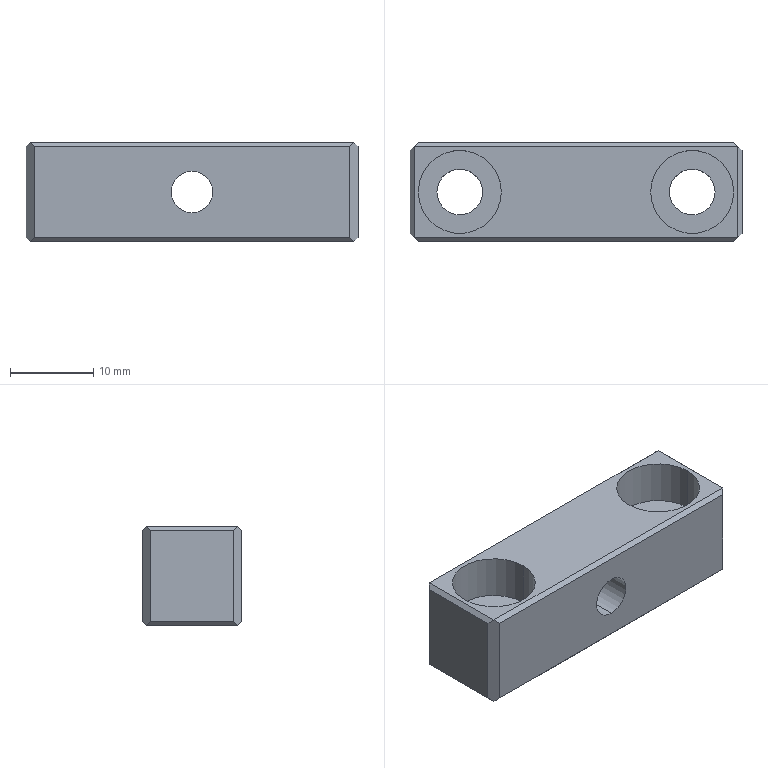Part | STEP file | 10000020605swp000-1 | 1 solid | 30 faces | box 40 x 12 x 12 mm | volume 4314 mm3 | plane 20 | cylinder 10 | commonest cylinder face diameters 5.5 x4 10 x4 5 x2
STEP:
#1=CARTESIAN_POINT('',(0.,6.,8.5));
#2=VERTEX_POINT('',#1);
#3=CARTESIAN_POINT('',(0.,6.,3.5));
#4=VERTEX_POINT('',#3);
#5=CARTESIAN_POINT('',(0.,6.,6.));
#6=DIRECTION('',(0.,-1.,0.));
#7=DIRECTION('',(0.,0.,-1.));
#8=AXIS2_PLACEMENT_3D('',#5,#6,#7);
#9=CIRCLE('',#8,2.5);
#10=EDGE_CURVE('',#2,#4,#9,.T.);
#11=ORIENTED_EDGE('',*,*,#10,.F.);
#12=CARTESIAN_POINT('',(0.,-6.,8.5));
#13=VERTEX_POINT('',#12);
#14=CARTESIAN_POINT('',(0.,-6.,8.5));
#15=DIRECTION('',(0.,-1.,0.));
#16=VECTOR('',#15,1000.);
#17=LINE('',#14,#16);
#18=EDGE_CURVE('',#2,#13,#17,.T.);
#19=ORIENTED_EDGE('',*,*,#18,.T.);
#20=CARTESIAN_POINT('',(0.,-6.,3.5));
#21=VERTEX_POINT('',#20);
#22=CARTESIAN_POINT('',(0.,-6.,6.));
#23=DIRECTION('',(0.,-1.,0.));
#24=DIRECTION('',(0.,0.,-1.));
#25=AXIS2_PLACEMENT_3D('',#22,#23,#24);
#26=CIRCLE('',#25,2.5);
#27=EDGE_CURVE('',#13,#21,#26,.T.);
#28=ORIENTED_EDGE('',*,*,#27,.T.);
#29=CARTESIAN_POINT('',(0.,-6.,3.5));
#30=DIRECTION('',(0.,-1.,0.));
#31=VECTOR('',#30,1000.);
#32=LINE('',#29,#31);
#33=EDGE_CURVE('',#4,#21,#32,.T.);
#34=ORIENTED_EDGE('',*,*,#33,.F.);
#35=EDGE_LOOP('',(#11,#19,#28,#34));
#36=FACE_OUTER_BOUND('',#35,.T.);
#37=CARTESIAN_POINT('',(0.,-6.,6.));
#38=DIRECTION('',(0.,-1.,0.));
#39=DIRECTION('',(0.,0.,-1.));
#40=AXIS2_PLACEMENT_3D('',#37,#38,#39);
#41=CYLINDRICAL_SURFACE('',#40,2.5);
#42=ADVANCED_FACE('',(#36),#41,.F.);
#43=CARTESIAN_POINT('',(-19.,0.,6.6));
#44=VERTEX_POINT('',#43);
#45=CARTESIAN_POINT('',(-9.,0.,6.6));
#46=VERTEX_POINT('',#45);
#47=CARTESIAN_POINT('',(-14.,0.,6.6));
#48=DIRECTION('',(0.,0.,1.));
#49=DIRECTION('',(1.,0.,0.));
#50=AXIS2_PLACEMENT_3D('',#47,#48,#49);
#51=CIRCLE('',#50,5.);
#52=EDGE_CURVE('',#44,#46,#51,.T.);
#53=ORIENTED_EDGE('',*,*,#52,.F.);
#54=CARTESIAN_POINT('',(-19.,0.,12.));
#55=VERTEX_POINT('',#54);
#56=CARTESIAN_POINT('',(-19.,0.,12.));
#57=DIRECTION('',(0.,0.,1.));
#58=VECTOR('',#57,1000.);
#59=LINE('',#56,#58);
#60=EDGE_CURVE('',#44,#55,#59,.T.);
#61=ORIENTED_EDGE('',*,*,#60,.T.);
#62=CARTESIAN_POINT('',(-9.,0.,12.));
#63=VERTEX_POINT('',#62);
#64=CARTESIAN_POINT('',(-14.,0.,12.));
#65=DIRECTION('',(0.,0.,1.));
#66=DIRECTION('',(1.,0.,0.));
#67=AXIS2_PLACEMENT_3D('',#64,#65,#66);
#68=CIRCLE('',#67,5.);
#69=EDGE_CURVE('',#55,#63,#68,.T.);
#70=ORIENTED_EDGE('',*,*,#69,.T.);
#71=CARTESIAN_POINT('',(-9.,0.,12.));
#72=DIRECTION('',(0.,0.,1.));
#73=VECTOR('',#72,1000.);
#74=LINE('',#71,#73);
#75=EDGE_CURVE('',#46,#63,#74,.T.);
#76=ORIENTED_EDGE('',*,*,#75,.F.);
#77=EDGE_LOOP('',(#53,#61,#70,#76));
#78=FACE_OUTER_BOUND('',#77,.T.);
#79=CARTESIAN_POINT('',(-14.,0.,12.));
#80=DIRECTION('',(0.,0.,1.));
#81=DIRECTION('',(1.,0.,0.));
#82=AXIS2_PLACEMENT_3D('',#79,#80,#81);
#83=CYLINDRICAL_SURFACE('',#82,5.);
#84=ADVANCED_FACE('',(#78),#83,.F.);
#85=CARTESIAN_POINT('',(-16.75,0.,0.));
#86=VERTEX_POINT('',#85);
#87=CARTESIAN_POINT('',(-11.25,0.,0.));
#88=VERTEX_POINT('',#87);
#89=CARTESIAN_POINT('',(-14.,0.,0.));
#90=DIRECTION('',(0.,0.,1.));
#91=DIRECTION('',(1.,0.,0.));
#92=AXIS2_PLACEMENT_3D('',#89,#90,#91);
#93=CIRCLE('',#92,2.75);
#94=EDGE_CURVE('',#86,#88,#93,.T.);
#95=ORIENTED_EDGE('',*,*,#94,.F.);
#96=CARTESIAN_POINT('',(-16.75,0.,6.6));
#97=VERTEX_POINT('',#96);
#98=CARTESIAN_POINT('',(-16.75,0.,12.));
#99=DIRECTION('',(0.,0.,1.));
#100=VECTOR('',#99,1000.);
#101=LINE('',#98,#100);
#102=EDGE_CURVE('',#86,#97,#101,.T.);
#103=ORIENTED_EDGE('',*,*,#102,.T.);
#104=CARTESIAN_POINT('',(-11.25,0.,6.6));
#105=VERTEX_POINT('',#104);
#106=CARTESIAN_POINT('',(-14.,0.,6.6));
#107=DIRECTION('',(0.,0.,1.));
#108=DIRECTION('',(1.,0.,0.));
#109=AXIS2_PLACEMENT_3D('',#106,#107,#108);
#110=CIRCLE('',#109,2.75);
#111=EDGE_CURVE('',#97,#105,#110,.T.);
#112=ORIENTED_EDGE('',*,*,#111,.T.);
#113=CARTESIAN_POINT('',(-11.25,0.,12.));
#114=DIRECTION('',(0.,0.,1.));
#115=VECTOR('',#114,1000.);
#116=LINE('',#113,#115);
#117=EDGE_CURVE('',#88,#105,#116,.T.);
#118=ORIENTED_EDGE('',*,*,#117,.F.);
#119=EDGE_LOOP('',(#95,#103,#112,#118));
#120=FACE_OUTER_BOUND('',#119,.T.);
#121=CARTESIAN_POINT('',(-14.,0.,12.));
#122=DIRECTION('',(0.,0.,1.));
#123=DIRECTION('',(1.,0.,0.));
#124=AXIS2_PLACEMENT_3D('',#121,#122,#123);
#125=CYLINDRICAL_SURFACE('',#124,2.75);
#126=ADVANCED_FACE('',(#120),#125,.F.);
#127=CARTESIAN_POINT('',(9.,0.,6.6));
#128=VERTEX_POINT('',#127);
#129=CARTESIAN_POINT('',(19.,0.,6.6));
#130=VERTEX_POINT('',#129);
#131=CARTESIAN_POINT('',(14.,0.,6.6));
#132=DIRECTION('',(0.,0.,1.));
#133=DIRECTION('',(1.,0.,0.));
#134=AXIS2_PLACEMENT_3D('',#131,#132,#133);
#135=CIRCLE('',#134,5.);
#136=EDGE_CURVE('',#128,#130,#135,.T.);
#137=ORIENTED_EDGE('',*,*,#136,.F.);
#138=CARTESIAN_POINT('',(9.,0.,12.));
#139=VERTEX_POINT('',#138);
#140=CARTESIAN_POINT('',(9.,0.,12.));
#141=DIRECTION('',(0.,0.,1.));
#142=VECTOR('',#141,1000.);
#143=LINE('',#140,#142);
#144=EDGE_CURVE('',#128,#139,#143,.T.);
#145=ORIENTED_EDGE('',*,*,#144,.T.);
#146=CARTESIAN_POINT('',(19.,0.,12.));
#147=VERTEX_POINT('',#146);
#148=CARTESIAN_POINT('',(14.,0.,12.));
#149=DIRECTION('',(0.,0.,1.));
#150=DIRECTION('',(1.,0.,0.));
#151=AXIS2_PLACEMENT_3D('',#148,#149,#150);
#152=CIRCLE('',#151,5.);
#153=EDGE_CURVE('',#139,#147,#152,.T.);
#154=ORIENTED_EDGE('',*,*,#153,.T.);
#155=CARTESIAN_POINT('',(19.,0.,12.));
#156=DIRECTION('',(0.,0.,1.));
#157=VECTOR('',#156,1000.);
#158=LINE('',#155,#157);
#159=EDGE_CURVE('',#130,#147,#158,.T.);
#160=ORIENTED_EDGE('',*,*,#159,.F.);
#161=EDGE_LOOP('',(#137,#145,#154,#160));
#162=FACE_OUTER_BOUND('',#161,.T.);
#163=CARTESIAN_POINT('',(14.,0.,12.));
#164=DIRECTION('',(0.,0.,1.));
#165=DIRECTION('',(1.,0.,0.));
#166=AXIS2_PLACEMENT_3D('',#163,#164,#165);
#167=CYLINDRICAL_SURFACE('',#166,5.);
#168=ADVANCED_FACE('',(#162),#167,.F.);
#169=CARTESIAN_POINT('',(11.25,0.,0.));
#170=VERTEX_POINT('',#169);
#171=CARTESIAN_POINT('',(16.75,0.,0.));
#172=VERTEX_POINT('',#171);
#173=CARTESIAN_POINT('',(14.,0.,0.));
#174=DIRECTION('',(0.,0.,1.));
#175=DIRECTION('',(1.,0.,0.));
#176=AXIS2_PLACEMENT_3D('',#173,#174,#175);
#177=CIRCLE('',#176,2.75);
#178=EDGE_CURVE('',#170,#172,#177,.T.);
#179=ORIENTED_EDGE('',*,*,#178,.F.);
#180=CARTESIAN_POINT('',(11.25,0.,6.6));
#181=VERTEX_POINT('',#180);
#182=CARTESIAN_POINT('',(11.25,0.,12.));
#183=DIRECTION('',(0.,0.,1.));
#184=VECTOR('',#183,1000.);
#185=LINE('',#182,#184);
#186=EDGE_CURVE('',#170,#181,#185,.T.);
#187=ORIENTED_EDGE('',*,*,#186,.T.);
#188=CARTESIAN_POINT('',(16.75,0.,6.6));
#189=VERTEX_POINT('',#188);
#190=CARTESIAN_POINT('',(14.,0.,6.6));
#191=DIRECTION('',(0.,0.,1.));
#192=DIRECTION('',(1.,0.,0.));
#193=AXIS2_PLACEMENT_3D('',#190,#191,#192);
#194=CIRCLE('',#193,2.75);
#195=EDGE_CURVE('',#181,#189,#194,.T.);
#196=ORIENTED_EDGE('',*,*,#195,.T.);
#197=CARTESIAN_POINT('',(16.75,0.,12.));
#198=DIRECTION('',(0.,0.,1.));
#199=VECTOR('',#198,1000.);
#200=LINE('',#197,#199);
#201=EDGE_CURVE('',#172,#189,#200,.T.);
#202=ORIENTED_EDGE('',*,*,#201,.F.);
#203=EDGE_LOOP('',(#179,#187,#196,#202));
#204=FACE_OUTER_BOUND('',#203,.T.);
#205=CARTESIAN_POINT('',(14.,0.,12.));
#206=DIRECTION('',(0.,0.,1.));
#207=DIRECTION('',(1.,0.,0.));
#208=AXIS2_PLACEMENT_3D('',#205,#206,#207);
#209=CYLINDRICAL_SURFACE('',#208,2.75);
#210=ADVANCED_FACE('',(#204),#209,.F.);
#211=CARTESIAN_POINT('',(-20.,5.,11.5));
#212=VERTEX_POINT('',#211);
#213=CARTESIAN_POINT('',(-20.,5.,0.5));
#214=VERTEX_POINT('',#213);
#215=CARTESIAN_POINT('',(-20.,5.,12.));
#216=DIRECTION('',(0.,0.,-1.));
#217=VECTOR('',#216,1000.);
#218=LINE('',#215,#217);
#219=EDGE_CURVE('',#212,#214,#218,.T.);
#220=ORIENTED_EDGE('',*,*,#219,.T.);
#221=CARTESIAN_POINT('',(-20.,-5.,0.5));
#222=VERTEX_POINT('',#221);
#223=CARTESIAN_POINT('',(-20.,6.,0.5));
#224=DIRECTION('',(0.,-1.,0.));
#225=VECTOR('',#224,1000.);
#226=LINE('',#223,#225);
#227=EDGE_CURVE('',#214,#222,#226,.T.);
#228=ORIENTED_EDGE('',*,*,#227,.T.);
#229=CARTESIAN_POINT('',(-20.,-5.,11.5));
#230=VERTEX_POINT('',#229);
#231=CARTESIAN_POINT('',(-20.,-5.,12.));
#232=DIRECTION('',(0.,0.,1.));
#233=VECTOR('',#232,1000.);
#234=LINE('',#231,#233);
#235=EDGE_CURVE('',#222,#230,#234,.T.);
#236=ORIENTED_EDGE('',*,*,#235,.T.);
#237=CARTESIAN_POINT('',(-20.,5.,11.5));
#238=DIRECTION('',(0.,1.,0.));
#239=VECTOR('',#238,1000.);
#240=LINE('',#237,#239);
#241=EDGE_CURVE('',#230,#212,#240,.T.);
#242=ORIENTED_EDGE('',*,*,#241,.T.);
#243=EDGE_LOOP('',(#220,#228,#236,#242));
#244=FACE_OUTER_BOUND('',#243,.T.);
#245=CARTESIAN_POINT('',(-20.,6.,12.));
#246=DIRECTION('',(1.,0.,0.));
#247=DIRECTION('',(0.,0.,-1.));
#248=AXIS2_PLACEMENT_3D('',#245,#246,#247);
#249=PLANE('',#248);
#250=ADVANCED_FACE('',(#244),#249,.F.);
#251=CARTESIAN_POINT('',(0.,-6.,6.));
#252=DIRECTION('',(0.,-1.,0.));
#253=DIRECTION('',(0.,0.,-1.));
#254=AXIS2_PLACEMENT_3D('',#251,#252,#253);
#255=CIRCLE('',#254,2.5);
#256=EDGE_CURVE('',#21,#13,#255,.T.);
#257=ORIENTED_EDGE('',*,*,#256,.F.);
#258=ORIENTED_EDGE('',*,*,#27,.F.);
#259=EDGE_LOOP('',(#257,#258));
#260=FACE_BOUND('',#259,.T.);
#261=CARTESIAN_POINT('',(-19.,-6.,11.5));
#262=VERTEX_POINT('',#261);
#263=CARTESIAN_POINT('',(-19.,-6.,0.5));
#264=VERTEX_POINT('',#263);
#265=CARTESIAN_POINT('',(-19.,-6.,12.));
#266=DIRECTION('',(0.,0.,-1.));
#267=VECTOR('',#266,1000.);
#268=LINE('',#265,#267);
#269=EDGE_CURVE('',#262,#264,#268,.T.);
#270=ORIENTED_EDGE('',*,*,#269,.T.);
#271=CARTESIAN_POINT('',(19.,-6.,0.5));
#272=VERTEX_POINT('',#271);
#273=CARTESIAN_POINT('',(-20.,-6.,0.5));
#274=DIRECTION('',(1.,0.,0.));
#275=VECTOR('',#274,1000.);
#276=LINE('',#273,#275);
#277=EDGE_CURVE('',#264,#272,#276,.T.);
#278=ORIENTED_EDGE('',*,*,#277,.T.);
#279=CARTESIAN_POINT('',(19.,-6.,11.5));
#280=VERTEX_POINT('',#279);
#281=CARTESIAN_POINT('',(19.,-6.,12.));
#282=DIRECTION('',(0.,0.,1.));
#283=VECTOR('',#282,1000.);
#284=LINE('',#281,#283);
#285=EDGE_CURVE('',#272,#280,#284,.T.);
#286=ORIENTED_EDGE('',*,*,#285,.T.);
#287=CARTESIAN_POINT('',(-19.,-6.,11.5));
#288=DIRECTION('',(-1.,0.,0.));
#289=VECTOR('',#288,1000.);
#290=LINE('',#287,#289);
#291=EDGE_CURVE('',#280,#262,#290,.T.);
#292=ORIENTED_EDGE('',*,*,#291,.T.);
#293=EDGE_LOOP('',(#270,#278,#286,#292));
#294=FACE_OUTER_BOUND('',#293,.T.);
#295=CARTESIAN_POINT('',(-20.,-6.,12.));
#296=DIRECTION('',(0.,1.,0.));
#297=DIRECTION('',(0.,0.,1.));
#298=AXIS2_PLACEMENT_3D('',#295,#296,#297);
#299=PLANE('',#298);
#300=ADVANCED_FACE('',(#260,#294),#299,.F.);
#301=CARTESIAN_POINT('',(20.,-5.,11.5));
#302=VERTEX_POINT('',#301);
#303=CARTESIAN_POINT('',(20.,-5.,0.5));
#304=VERTEX_POINT('',#303);
#305=CARTESIAN_POINT('',(20.,-5.,12.));
#306=DIRECTION('',(0.,0.,-1.));
#307=VECTOR('',#306,1000.);
#308=LINE('',#305,#307);
#309=EDGE_CURVE('',#302,#304,#308,.T.);
#310=ORIENTED_EDGE('',*,*,#309,.T.);
#311=CARTESIAN_POINT('',(20.,5.,0.5));
#312=VERTEX_POINT('',#311);
#313=CARTESIAN_POINT('',(20.,6.,0.5));
#314=DIRECTION('',(0.,1.,0.));
#315=VECTOR('',#314,1000.);
#316=LINE('',#313,#315);
#317=EDGE_CURVE('',#304,#312,#316,.T.);
#318=ORIENTED_EDGE('',*,*,#317,.T.);
#319=CARTESIAN_POINT('',(20.,5.,11.5));
#320=VERTEX_POINT('',#319);
#321=CARTESIAN_POINT('',(20.,5.,12.));
#322=DIRECTION('',(0.,0.,1.));
#323=VECTOR('',#322,1000.);
#324=LINE('',#321,#323);
#325=EDGE_CURVE('',#312,#320,#324,.T.);
#326=ORIENTED_EDGE('',*,*,#325,.T.);
#327=CARTESIAN_POINT('',(20.,-5.,11.5));
#328=DIRECTION('',(0.,-1.,0.));
#329=VECTOR('',#328,1000.);
#330=LINE('',#327,#329);
#331=EDGE_CURVE('',#320,#302,#330,.T.);
#332=ORIENTED_EDGE('',*,*,#331,.T.);
#333=EDGE_LOOP('',(#310,#318,#326,#332));
#334=FACE_OUTER_BOUND('',#333,.T.);
#335=CARTESIAN_POINT('',(20.,6.,12.));
#336=DIRECTION('',(-1.,0.,0.));
#337=DIRECTION('',(0.,0.,1.));
#338=AXIS2_PLACEMENT_3D('',#335,#336,#337);
#339=PLANE('',#338);
#340=ADVANCED_FACE('',(#334),#339,.F.);
#341=CARTESIAN_POINT('',(0.,6.,6.));
#342=DIRECTION('',(0.,-1.,0.));
#343=DIRECTION('',(0.,0.,-1.));
#344=AXIS2_PLACEMENT_3D('',#341,#342,#343);
#345=CIRCLE('',#344,2.5);
#346=EDGE_CURVE('',#4,#2,#345,.T.);
#347=ORIENTED_EDGE('',*,*,#346,.T.);
#348=ORIENTED_EDGE('',*,*,#10,.T.);
#349=EDGE_LOOP('',(#347,#348));
#350=FACE_BOUND('',#349,.T.);
#351=CARTESIAN_POINT('',(19.,6.,11.5));
#352=VERTEX_POINT('',#351);
#353=CARTESIAN_POINT('',(19.,6.,0.5));
#354=VERTEX_POINT('',#353);
#355=CARTESIAN_POINT('',(19.,6.,12.));
#356=DIRECTION('',(0.,0.,-1.));
#357=VECTOR('',#356,1000.);
#358=LINE('',#355,#357);
#359=EDGE_CURVE('',#352,#354,#358,.T.);
#360=ORIENTED_EDGE('',*,*,#359,.T.);
#361=CARTESIAN_POINT('',(-19.,6.,0.5));
#362=VERTEX_POINT('',#361);
#363=CARTESIAN_POINT('',(-20.,6.,0.5));
#364=DIRECTION('',(-1.,0.,0.));
#365=VECTOR('',#364,1000.);
#366=LINE('',#363,#365);
#367=EDGE_CURVE('',#354,#362,#366,.T.);
#368=ORIENTED_EDGE('',*,*,#367,.T.);
#369=CARTESIAN_POINT('',(-19.,6.,11.5));
#370=VERTEX_POINT('',#369);
#371=CARTESIAN_POINT('',(-19.,6.,12.));
#372=DIRECTION('',(0.,0.,1.));
#373=VECTOR('',#372,1000.);
#374=LINE('',#371,#373);
#375=EDGE_CURVE('',#362,#370,#374,.T.);
#376=ORIENTED_EDGE('',*,*,#375,.T.);
#377=CARTESIAN_POINT('',(19.,6.,11.5));
#378=DIRECTION('',(1.,0.,0.));
#379=VECTOR('',#378,1000.);
#380=LINE('',#377,#379);
#381=EDGE_CURVE('',#370,#352,#380,.T.);
#382=ORIENTED_EDGE('',*,*,#381,.T.);
#383=EDGE_LOOP('',(#360,#368,#376,#382));
#384=FACE_OUTER_BOUND('',#383,.T.);
#385=CARTESIAN_POINT('',(-20.,6.,12.));
#386=DIRECTION('',(0.,-1.,0.));
#387=DIRECTION('',(0.,0.,-1.));
#388=AXIS2_PLACEMENT_3D('',#385,#386,#387);
#389=PLANE('',#388);
#390=ADVANCED_FACE('',(#350,#384),#389,.F.);
#391=CARTESIAN_POINT('',(-14.,0.,12.));
#392=DIRECTION('',(0.,0.,1.));
#393=DIRECTION('',(1.,0.,0.));
#394=AXIS2_PLACEMENT_3D('',#391,#392,#393);
#395=CIRCLE('',#394,5.);
#396=EDGE_CURVE('',#63,#55,#395,.T.);
#397=ORIENTED_EDGE('',*,*,#396,.F.);
#398=ORIENTED_EDGE('',*,*,#69,.F.);
#399=EDGE_LOOP('',(#397,#398));
#400=FACE_BOUND('',#399,.T.);
#401=CARTESIAN_POINT('',(14.,0.,12.));
#402=DIRECTION('',(0.,0.,1.));
#403=DIRECTION('',(1.,0.,0.));
#404=AXIS2_PLACEMENT_3D('',#401,#402,#403);
#405=CIRCLE('',#404,5.);
#406=EDGE_CURVE('',#147,#139,#405,.T.);
#407=ORIENTED_EDGE('',*,*,#406,.F.);
#408=ORIENTED_EDGE('',*,*,#153,.F.);
#409=EDGE_LOOP('',(#407,#408));
#410=FACE_BOUND('',#409,.T.);
#411=CARTESIAN_POINT('',(19.5,5.5,12.));
#412=VERTEX_POINT('',#411);
#413=CARTESIAN_POINT('',(-19.5,5.5,12.));
#414=VERTEX_POINT('',#413);
#415=CARTESIAN_POINT('',(-19.,5.5,12.));
#416=DIRECTION('',(-1.,0.,0.));
#417=VECTOR('',#416,1000.);
#418=LINE('',#415,#417);
#419=EDGE_CURVE('',#412,#414,#418,.T.);
#420=ORIENTED_EDGE('',*,*,#419,.T.);
#421=CARTESIAN_POINT('',(-19.5,-5.5,12.));
#422=VERTEX_POINT('',#421);
#423=CARTESIAN_POINT('',(-19.5,-5.,12.));
#424=DIRECTION('',(0.,-1.,0.));
#425=VECTOR('',#424,1000.);
#426=LINE('',#423,#425);
#427=EDGE_CURVE('',#414,#422,#426,.T.);
#428=ORIENTED_EDGE('',*,*,#427,.T.);
#429=CARTESIAN_POINT('',(19.5,-5.5,12.));
#430=VERTEX_POINT('',#429);
#431=CARTESIAN_POINT('',(19.,-5.5,12.));
#432=DIRECTION('',(1.,0.,0.));
#433=VECTOR('',#432,1000.);
#434=LINE('',#431,#433);
#435=EDGE_CURVE('',#422,#430,#434,.T.);
#436=ORIENTED_EDGE('',*,*,#435,.T.);
#437=CARTESIAN_POINT('',(19.5,5.,12.));
#438=DIRECTION('',(0.,1.,0.));
#439=VECTOR('',#438,1000.);
#440=LINE('',#437,#439);
#441=EDGE_CURVE('',#430,#412,#440,.T.);
#442=ORIENTED_EDGE('',*,*,#441,.T.);
#443=EDGE_LOOP('',(#420,#428,#436,#442));
#444=FACE_OUTER_BOUND('',#443,.T.);
#445=CARTESIAN_POINT('',(0.,0.,12.));
#446=DIRECTION('',(0.,0.,1.));
#447=DIRECTION('',(1.,0.,0.));
#448=AXIS2_PLACEMENT_3D('',#445,#446,#447);
#449=PLANE('',#448);
#450=ADVANCED_FACE('',(#400,#410,#444),#449,.T.);
#451=CARTESIAN_POINT('',(-14.,0.,0.));
#452=DIRECTION('',(0.,0.,1.));
#453=DIRECTION('',(1.,0.,0.));
#454=AXIS2_PLACEMENT_3D('',#451,#452,#453);
#455=CIRCLE('',#454,2.75);
#456=EDGE_CURVE('',#88,#86,#455,.T.);
#457=ORIENTED_EDGE('',*,*,#456,.T.);
#458=ORIENTED_EDGE('',*,*,#94,.T.);
#459=EDGE_LOOP('',(#457,#458));
#460=FACE_BOUND('',#459,.T.);
#461=CARTESIAN_POINT('',(14.,0.,0.));
#462=DIRECTION('',(0.,0.,1.));
#463=DIRECTION('',(1.,0.,0.));
#464=AXIS2_PLACEMENT_3D('',#461,#462,#463);
#465=CIRCLE('',#464,2.75);
#466=EDGE_CURVE('',#172,#170,#465,.T.);
#467=ORIENTED_EDGE('',*,*,#466,.T.);
#468=ORIENTED_EDGE('',*,*,#178,.T.);
#469=EDGE_LOOP('',(#467,#468));
#470=FACE_BOUND('',#469,.T.);
#471=CARTESIAN_POINT('',(19.5,5.5,0.));
#472=VERTEX_POINT('',#471);
#473=CARTESIAN_POINT('',(19.5,-5.5,0.));
#474=VERTEX_POINT('',#473);
#475=CARTESIAN_POINT('',(19.5,0.,0.));
#476=DIRECTION('',(0.,-1.,0.));
#477=VECTOR('',#476,1000.);
#478=LINE('',#475,#477);
#479=EDGE_CURVE('',#472,#474,#478,.T.);
#480=ORIENTED_EDGE('',*,*,#479,.T.);
#481=CARTESIAN_POINT('',(-19.5,-5.5,0.));
#482=VERTEX_POINT('',#481);
#483=CARTESIAN_POINT('',(0.,-5.5,0.));
#484=DIRECTION('',(-1.,0.,0.));
#485=VECTOR('',#484,1000.);
#486=LINE('',#483,#485);
#487=EDGE_CURVE('',#474,#482,#486,.T.);
#488=ORIENTED_EDGE('',*,*,#487,.T.);
#489=CARTESIAN_POINT('',(-19.5,5.5,0.));
#490=VERTEX_POINT('',#489);
#491=CARTESIAN_POINT('',(-19.5,0.,0.));
#492=DIRECTION('',(0.,1.,0.));
#493=VECTOR('',#492,1000.);
#494=LINE('',#491,#493);
#495=EDGE_CURVE('',#482,#490,#494,.T.);
#496=ORIENTED_EDGE('',*,*,#495,.T.);
#497=CARTESIAN_POINT('',(0.,5.5,0.));
#498=DIRECTION('',(1.,0.,0.));
#499=VECTOR('',#498,1000.);
#500=LINE('',#497,#499);
#501=EDGE_CURVE('',#490,#472,#500,.T.);
#502=ORIENTED_EDGE('',*,*,#501,.T.);
#503=EDGE_LOOP('',(#480,#488,#496,#502));
#504=FACE_OUTER_BOUND('',#503,.T.);
#505=CARTESIAN_POINT('',(0.,0.,0.));
#506=DIRECTION('',(0.,0.,1.));
#507=DIRECTION('',(1.,0.,0.));
#508=AXIS2_PLACEMENT_3D('',#505,#506,#507);
#509=PLANE('',#508);
#510=ADVANCED_FACE('',(#460,#470,#504),#509,.F.);
#511=ORIENTED_EDGE('',*,*,#186,.F.);
#512=ORIENTED_EDGE('',*,*,#466,.F.);
#513=ORIENTED_EDGE('',*,*,#201,.T.);
#514=CARTESIAN_POINT('',(14.,0.,6.6));
#515=DIRECTION('',(0.,0.,1.));
#516=DIRECTION('',(1.,0.,0.));
#517=AXIS2_PLACEMENT_3D('',#514,#515,#516);
#518=CIRCLE('',#517,2.75);
#519=EDGE_CURVE('',#189,#181,#518,.T.);
#520=ORIENTED_EDGE('',*,*,#519,.T.);
#521=EDGE_LOOP('',(#511,#512,#513,#520));
#522=FACE_OUTER_BOUND('',#521,.T.);
#523=CARTESIAN_POINT('',(14.,0.,12.));
#524=DIRECTION('',(0.,0.,1.));
#525=DIRECTION('',(1.,0.,0.));
#526=AXIS2_PLACEMENT_3D('',#523,#524,#525);
#527=CYLINDRICAL_SURFACE('',#526,2.75);
#528=ADVANCED_FACE('',(#522),#527,.F.);
#529=ORIENTED_EDGE('',*,*,#519,.F.);
#530=ORIENTED_EDGE('',*,*,#195,.F.);
#531=EDGE_LOOP('',(#529,#530));
#532=FACE_BOUND('',#531,.T.);
#533=CARTESIAN_POINT('',(14.,0.,6.6));
#534=DIRECTION('',(0.,0.,1.));
#535=DIRECTION('',(1.,0.,0.));
#536=AXIS2_PLACEMENT_3D('',#533,#534,#535);
#537=CIRCLE('',#536,5.);
#538=EDGE_CURVE('',#130,#128,#537,.T.);
#539=ORIENTED_EDGE('',*,*,#538,.T.);
#540=ORIENTED_EDGE('',*,*,#136,.T.);
#541=EDGE_LOOP('',(#539,#540));
#542=FACE_OUTER_BOUND('',#541,.T.);
#543=CARTESIAN_POINT('',(16.75,0.,6.6));
#544=DIRECTION('',(0.,0.,-1.));
#545=DIRECTION('',(-1.,0.,0.));
#546=AXIS2_PLACEMENT_3D('',#543,#544,#545);
#547=PLANE('',#546);
#548=ADVANCED_FACE('',(#532,#542),#547,.F.);
#549=ORIENTED_EDGE('',*,*,#144,.F.);
#550=ORIENTED_EDGE('',*,*,#538,.F.);
#551=ORIENTED_EDGE('',*,*,#159,.T.);
#552=ORIENTED_EDGE('',*,*,#406,.T.);
#553=EDGE_LOOP('',(#549,#550,#551,#552));
#554=FACE_OUTER_BOUND('',#553,.T.);
#555=CARTESIAN_POINT('',(14.,0.,12.));
#556=DIRECTION('',(0.,0.,1.));
#557=DIRECTION('',(1.,0.,0.));
#558=AXIS2_PLACEMENT_3D('',#555,#556,#557);
#559=CYLINDRICAL_SURFACE('',#558,5.);
#560=ADVANCED_FACE('',(#554),#559,.F.);
#561=ORIENTED_EDGE('',*,*,#102,.F.);
#562=ORIENTED_EDGE('',*,*,#456,.F.);
#563=ORIENTED_EDGE('',*,*,#117,.T.);
#564=CARTESIAN_POINT('',(-14.,0.,6.6));
#565=DIRECTION('',(0.,0.,1.));
#566=DIRECTION('',(1.,0.,0.));
#567=AXIS2_PLACEMENT_3D('',#564,#565,#566);
#568=CIRCLE('',#567,2.75);
#569=EDGE_CURVE('',#105,#97,#568,.T.);
#570=ORIENTED_EDGE('',*,*,#569,.T.);
#571=EDGE_LOOP('',(#561,#562,#563,#570));
#572=FACE_OUTER_BOUND('',#571,.T.);
#573=CARTESIAN_POINT('',(-14.,0.,12.));
#574=DIRECTION('',(0.,0.,1.));
#575=DIRECTION('',(1.,0.,0.));
#576=AXIS2_PLACEMENT_3D('',#573,#574,#575);
#577=CYLINDRICAL_SURFACE('',#576,2.75);
#578=ADVANCED_FACE('',(#572),#577,.F.);
#579=ORIENTED_EDGE('',*,*,#569,.F.);
#580=ORIENTED_EDGE('',*,*,#111,.F.);
#581=EDGE_LOOP('',(#579,#580));
#582=FACE_BOUND('',#581,.T.);
#583=CARTESIAN_POINT('',(-14.,0.,6.6));
#584=DIRECTION('',(0.,0.,1.));
#585=DIRECTION('',(1.,0.,0.));
#586=AXIS2_PLACEMENT_3D('',#583,#584,#585);
#587=CIRCLE('',#586,5.);
#588=EDGE_CURVE('',#46,#44,#587,.T.);
#589=ORIENTED_EDGE('',*,*,#588,.T.);
#590=ORIENTED_EDGE('',*,*,#52,.T.);
#591=EDGE_LOOP('',(#589,#590));
#592=FACE_OUTER_BOUND('',#591,.T.);
#593=CARTESIAN_POINT('',(-11.25,0.,6.6));
#594=DIRECTION('',(0.,0.,-1.));
#595=DIRECTION('',(-1.,0.,0.));
#596=AXIS2_PLACEMENT_3D('',#593,#594,#595);
#597=PLANE('',#596);
#598=ADVANCED_FACE('',(#582,#592),#597,.F.);
#599=ORIENTED_EDGE('',*,*,#60,.F.);
#600=ORIENTED_EDGE('',*,*,#588,.F.);
#601=ORIENTED_EDGE('',*,*,#75,.T.);
#602=ORIENTED_EDGE('',*,*,#396,.T.);
#603=EDGE_LOOP('',(#599,#600,#601,#602));
#604=FACE_OUTER_BOUND('',#603,.T.);
#605=CARTESIAN_POINT('',(-14.,0.,12.));
#606=DIRECTION('',(0.,0.,1.));
#607=DIRECTION('',(1.,0.,0.));
#608=AXIS2_PLACEMENT_3D('',#605,#606,#607);
#609=CYLINDRICAL_SURFACE('',#608,5.);
#610=ADVANCED_FACE('',(#604),#609,.F.);
#611=ORIENTED_EDGE('',*,*,#18,.F.);
#612=ORIENTED_EDGE('',*,*,#346,.F.);
#613=ORIENTED_EDGE('',*,*,#33,.T.);
#614=ORIENTED_EDGE('',*,*,#256,.T.);
#615=EDGE_LOOP('',(#611,#612,#613,#614));
#616=FACE_OUTER_BOUND('',#615,.T.);
#617=CARTESIAN_POINT('',(0.,-6.,6.));
#618=DIRECTION('',(0.,-1.,0.));
#619=DIRECTION('',(0.,0.,-1.));
#620=AXIS2_PLACEMENT_3D('',#617,#618,#619);
#621=CYLINDRICAL_SURFACE('',#620,2.5);
#622=ADVANCED_FACE('',(#616),#621,.F.);
#623=ORIENTED_EDGE('',*,*,#285,.F.);
#624=CARTESIAN_POINT('',(15.833,-9.167,3.667));
#625=DIRECTION('',(0.5774,0.5774,-0.5774));
#626=VECTOR('',#625,1000.);
#627=LINE('',#624,#626);
#628=EDGE_CURVE('',#272,#474,#627,.T.);
#629=ORIENTED_EDGE('',*,*,#628,.T.);
#630=CARTESIAN_POINT('',(23.833,-1.167,4.333));
#631=DIRECTION('',(0.5774,0.5774,0.5774));
#632=VECTOR('',#631,1000.);
#633=LINE('',#630,#632);
#634=EDGE_CURVE('',#474,#304,#633,.T.);
#635=ORIENTED_EDGE('',*,*,#634,.T.);
#636=ORIENTED_EDGE('',*,*,#309,.F.);
#637=CARTESIAN_POINT('',(19.833,-5.167,11.667));
#638=DIRECTION('',(-0.5774,-0.5774,0.5774));
#639=VECTOR('',#638,1000.);
#640=LINE('',#637,#639);
#641=EDGE_CURVE('',#302,#430,#640,.T.);
#642=ORIENTED_EDGE('',*,*,#641,.T.);
#643=CARTESIAN_POINT('',(19.833,-5.167,12.333));
#644=DIRECTION('',(-0.5774,-0.5774,-0.5774));
#645=VECTOR('',#644,1000.);
#646=LINE('',#643,#645);
#647=EDGE_CURVE('',#430,#280,#646,.T.);
#648=ORIENTED_EDGE('',*,*,#647,.T.);
#649=EDGE_LOOP('',(#623,#629,#635,#636,#642,#648));
#650=FACE_OUTER_BOUND('',#649,.T.);
#651=CARTESIAN_POINT('',(20.,-5.,12.));
#652=DIRECTION('',(-0.7071,0.7071,0.));
#653=DIRECTION('',(0.,0.,-1.));
#654=AXIS2_PLACEMENT_3D('',#651,#652,#653);
#655=PLANE('',#654);
#656=ADVANCED_FACE('',(#650),#655,.F.);
#657=ORIENTED_EDGE('',*,*,#325,.F.);
#658=CARTESIAN_POINT('',(23.167,1.833,3.667));
#659=DIRECTION('',(-0.5774,0.5774,-0.5774));
#660=VECTOR('',#659,1000.);
#661=LINE('',#658,#660);
#662=EDGE_CURVE('',#312,#472,#661,.T.);
#663=ORIENTED_EDGE('',*,*,#662,.T.);
#664=CARTESIAN_POINT('',(15.167,9.833,4.333));
#665=DIRECTION('',(-0.5774,0.5774,0.5774));
#666=VECTOR('',#665,1000.);
#667=LINE('',#664,#666);
#668=EDGE_CURVE('',#472,#354,#667,.T.);
#669=ORIENTED_EDGE('',*,*,#668,.T.);
#670=ORIENTED_EDGE('',*,*,#359,.F.);
#671=CARTESIAN_POINT('',(19.167,5.833,11.667));
#672=DIRECTION('',(0.5774,-0.5774,0.5774));
#673=VECTOR('',#672,1000.);
#674=LINE('',#671,#673);
#675=EDGE_CURVE('',#352,#412,#674,.T.);
#676=ORIENTED_EDGE('',*,*,#675,.T.);
#677=CARTESIAN_POINT('',(19.167,5.833,12.333));
#678=DIRECTION('',(0.5774,-0.5774,-0.5774));
#679=VECTOR('',#678,1000.);
#680=LINE('',#677,#679);
#681=EDGE_CURVE('',#412,#320,#680,.T.);
#682=ORIENTED_EDGE('',*,*,#681,.T.);
#683=EDGE_LOOP('',(#657,#663,#669,#670,#676,#682));
#684=FACE_OUTER_BOUND('',#683,.T.);
#685=CARTESIAN_POINT('',(19.,6.,12.));
#686=DIRECTION('',(-0.7071,-0.7071,0.));
#687=DIRECTION('',(0.,0.,-1.));
#688=AXIS2_PLACEMENT_3D('',#685,#686,#687);
#689=PLANE('',#688);
#690=ADVANCED_FACE('',(#684),#689,.F.);
#691=CARTESIAN_POINT('',(-23.167,-1.833,3.667));
#692=DIRECTION('',(0.5774,-0.5774,-0.5774));
#693=VECTOR('',#692,1000.);
#694=LINE('',#691,#693);
#695=EDGE_CURVE('',#222,#482,#694,.T.);
#696=ORIENTED_EDGE('',*,*,#695,.T.);
#697=CARTESIAN_POINT('',(-15.167,-9.833,4.333));
#698=DIRECTION('',(0.5774,-0.5774,0.5774));
#699=VECTOR('',#698,1000.);
#700=LINE('',#697,#699);
#701=EDGE_CURVE('',#482,#264,#700,.T.);
#702=ORIENTED_EDGE('',*,*,#701,.T.);
#703=ORIENTED_EDGE('',*,*,#269,.F.);
#704=CARTESIAN_POINT('',(-19.167,-5.833,11.667));
#705=DIRECTION('',(-0.5774,0.5774,0.5774));
#706=VECTOR('',#705,1000.);
#707=LINE('',#704,#706);
#708=EDGE_CURVE('',#262,#422,#707,.T.);
#709=ORIENTED_EDGE('',*,*,#708,.T.);
#710=CARTESIAN_POINT('',(-19.167,-5.833,12.333));
#711=DIRECTION('',(-0.5774,0.5774,-0.5774));
#712=VECTOR('',#711,1000.);
#713=LINE('',#710,#712);
#714=EDGE_CURVE('',#422,#230,#713,.T.);
#715=ORIENTED_EDGE('',*,*,#714,.T.);
#716=ORIENTED_EDGE('',*,*,#235,.F.);
#717=EDGE_LOOP('',(#696,#702,#703,#709,#715,#716));
#718=FACE_OUTER_BOUND('',#717,.T.);
#719=CARTESIAN_POINT('',(-19.,-6.,12.));
#720=DIRECTION('',(0.7071,0.7071,0.));
#721=DIRECTION('',(0.,0.,-1.));
#722=AXIS2_PLACEMENT_3D('',#719,#720,#721);
#723=PLANE('',#722);
#724=ADVANCED_FACE('',(#718),#723,.F.);
#725=CARTESIAN_POINT('',(-15.833,9.167,3.667));
#726=DIRECTION('',(-0.5774,-0.5774,-0.5774));
#727=VECTOR('',#726,1000.);
#728=LINE('',#725,#727);
#729=EDGE_CURVE('',#362,#490,#728,.T.);
#730=ORIENTED_EDGE('',*,*,#729,.T.);
#731=CARTESIAN_POINT('',(-23.833,1.167,4.333));
#732=DIRECTION('',(-0.5774,-0.5774,0.5774));
#733=VECTOR('',#732,1000.);
#734=LINE('',#731,#733);
#735=EDGE_CURVE('',#490,#214,#734,.T.);
#736=ORIENTED_EDGE('',*,*,#735,.T.);
#737=ORIENTED_EDGE('',*,*,#219,.F.);
#738=CARTESIAN_POINT('',(-19.833,5.167,11.667));
#739=DIRECTION('',(0.5774,0.5774,0.5774));
#740=VECTOR('',#739,1000.);
#741=LINE('',#738,#740);
#742=EDGE_CURVE('',#212,#414,#741,.T.);
#743=ORIENTED_EDGE('',*,*,#742,.T.);
#744=CARTESIAN_POINT('',(-19.833,5.167,12.333));
#745=DIRECTION('',(0.5774,0.5774,-0.5774));
#746=VECTOR('',#745,1000.);
#747=LINE('',#744,#746);
#748=EDGE_CURVE('',#414,#370,#747,.T.);
#749=ORIENTED_EDGE('',*,*,#748,.T.);
#750=ORIENTED_EDGE('',*,*,#375,.F.);
#751=EDGE_LOOP('',(#730,#736,#737,#743,#749,#750));
#752=FACE_OUTER_BOUND('',#751,.T.);
#753=CARTESIAN_POINT('',(-20.,5.,12.));
#754=DIRECTION('',(0.7071,-0.7071,0.));
#755=DIRECTION('',(0.,0.,-1.));
#756=AXIS2_PLACEMENT_3D('',#753,#754,#755);
#757=PLANE('',#756);
#758=ADVANCED_FACE('',(#752),#757,.F.);
#759=ORIENTED_EDGE('',*,*,#701,.F.);
#760=ORIENTED_EDGE('',*,*,#487,.F.);
#761=ORIENTED_EDGE('',*,*,#628,.F.);
#762=ORIENTED_EDGE('',*,*,#277,.F.);
#763=EDGE_LOOP('',(#759,#760,#761,#762));
#764=FACE_OUTER_BOUND('',#763,.T.);
#765=CARTESIAN_POINT('',(-20.,-6.,0.5));
#766=DIRECTION('',(0.,0.7071,0.7071));
#767=DIRECTION('',(1.,0.,0.));
#768=AXIS2_PLACEMENT_3D('',#765,#766,#767);
#769=PLANE('',#768);
#770=ADVANCED_FACE('',(#764),#769,.F.);
#771=ORIENTED_EDGE('',*,*,#634,.F.);
#772=ORIENTED_EDGE('',*,*,#479,.F.);
#773=ORIENTED_EDGE('',*,*,#662,.F.);
#774=ORIENTED_EDGE('',*,*,#317,.F.);
#775=EDGE_LOOP('',(#771,#772,#773,#774));
#776=FACE_OUTER_BOUND('',#775,.T.);
#777=CARTESIAN_POINT('',(20.,6.,0.5));
#778=DIRECTION('',(-0.7071,0.,0.7071));
#779=DIRECTION('',(0.,1.,0.));
#780=AXIS2_PLACEMENT_3D('',#777,#778,#779);
#781=PLANE('',#780);
#782=ADVANCED_FACE('',(#776),#781,.F.);
#783=ORIENTED_EDGE('',*,*,#735,.F.);
#784=ORIENTED_EDGE('',*,*,#495,.F.);
#785=ORIENTED_EDGE('',*,*,#695,.F.);
#786=ORIENTED_EDGE('',*,*,#227,.F.);
#787=EDGE_LOOP('',(#783,#784,#785,#786));
#788=FACE_OUTER_BOUND('',#787,.T.);
#789=CARTESIAN_POINT('',(-20.,6.,0.5));
#790=DIRECTION('',(0.7071,0.,0.7071));
#791=DIRECTION('',(0.,-1.,0.));
#792=AXIS2_PLACEMENT_3D('',#789,#790,#791);
#793=PLANE('',#792);
#794=ADVANCED_FACE('',(#788),#793,.F.);
#795=ORIENTED_EDGE('',*,*,#668,.F.);
#796=ORIENTED_EDGE('',*,*,#501,.F.);
#797=ORIENTED_EDGE('',*,*,#729,.F.);
#798=ORIENTED_EDGE('',*,*,#367,.F.);
#799=EDGE_LOOP('',(#795,#796,#797,#798));
#800=FACE_OUTER_BOUND('',#799,.T.);
#801=CARTESIAN_POINT('',(-20.,6.,0.5));
#802=DIRECTION('',(0.,-0.7071,0.7071));
#803=DIRECTION('',(-1.,0.,0.));
#804=AXIS2_PLACEMENT_3D('',#801,#802,#803);
#805=PLANE('',#804);
#806=ADVANCED_FACE('',(#800),#805,.F.);
#807=ORIENTED_EDGE('',*,*,#742,.F.);
#808=ORIENTED_EDGE('',*,*,#241,.F.);
#809=ORIENTED_EDGE('',*,*,#714,.F.);
#810=ORIENTED_EDGE('',*,*,#427,.F.);
#811=EDGE_LOOP('',(#807,#808,#809,#810));
#812=FACE_OUTER_BOUND('',#811,.T.);
#813=CARTESIAN_POINT('',(-19.5,0.,12.));
#814=DIRECTION('',(-0.7071,0.,0.7071));
#815=DIRECTION('',(0.,1.,0.));
#816=AXIS2_PLACEMENT_3D('',#813,#814,#815);
#817=PLANE('',#816);
#818=ADVANCED_FACE('',(#812),#817,.T.);
#819=ORIENTED_EDGE('',*,*,#708,.F.);
#820=ORIENTED_EDGE('',*,*,#291,.F.);
#821=ORIENTED_EDGE('',*,*,#647,.F.);
#822=ORIENTED_EDGE('',*,*,#435,.F.);
#823=EDGE_LOOP('',(#819,#820,#821,#822));
#824=FACE_OUTER_BOUND('',#823,.T.);
#825=CARTESIAN_POINT('',(0.,-5.5,12.));
#826=DIRECTION('',(0.,-0.7071,0.7071));
#827=DIRECTION('',(-1.,0.,0.));
#828=AXIS2_PLACEMENT_3D('',#825,#826,#827);
#829=PLANE('',#828);
#830=ADVANCED_FACE('',(#824),#829,.T.);
#831=ORIENTED_EDGE('',*,*,#675,.F.);
#832=ORIENTED_EDGE('',*,*,#381,.F.);
#833=ORIENTED_EDGE('',*,*,#748,.F.);
#834=ORIENTED_EDGE('',*,*,#419,.F.);
#835=EDGE_LOOP('',(#831,#832,#833,#834));
#836=FACE_OUTER_BOUND('',#835,.T.);
#837=CARTESIAN_POINT('',(0.,5.5,12.));
#838=DIRECTION('',(0.,0.7071,0.7071));
#839=DIRECTION('',(1.,0.,0.));
#840=AXIS2_PLACEMENT_3D('',#837,#838,#839);
#841=PLANE('',#840);
#842=ADVANCED_FACE('',(#836),#841,.T.);
#843=ORIENTED_EDGE('',*,*,#641,.F.);
#844=ORIENTED_EDGE('',*,*,#331,.F.);
#845=ORIENTED_EDGE('',*,*,#681,.F.);
#846=ORIENTED_EDGE('',*,*,#441,.F.);
#847=EDGE_LOOP('',(#843,#844,#845,#846));
#848=FACE_OUTER_BOUND('',#847,.T.);
#849=CARTESIAN_POINT('',(19.5,0.,12.));
#850=DIRECTION('',(0.7071,0.,0.7071));
#851=DIRECTION('',(0.,-1.,0.));
#852=AXIS2_PLACEMENT_3D('',#849,#850,#851);
#853=PLANE('',#852);
#854=ADVANCED_FACE('',(#848),#853,.T.);
#855=CLOSED_SHELL('',(#42,#84,#126,#168,#210,#250,#300,#340,#390,#450,#510,#528,#548,#560,#578,#598,#610,#622,#656,#690,#724,#758,#770,#782,#794,#806,#818,#830,#842,#854));
#856=MANIFOLD_SOLID_BREP('',#855);
#857=CARTESIAN_POINT('',(0.,0.,0.));
#858=DIRECTION('',(0.,0.,1.));
#859=DIRECTION('',(1.,0.,0.));
#860=AXIS2_PLACEMENT_3D('',#857,#858,#859);
#861=(LENGTH_UNIT()NAMED_UNIT(*)SI_UNIT(.MILLI.,.METRE.));
#862=UNCERTAINTY_MEASURE_WITH_UNIT(LENGTH_MEASURE(0.00001),#861,'','');
#863=(NAMED_UNIT(*)PLANE_ANGLE_UNIT()SI_UNIT($,.RADIAN.));
#864=(NAMED_UNIT(*)SI_UNIT($,.STERADIAN.)SOLID_ANGLE_UNIT());
#865=(GEOMETRIC_REPRESENTATION_CONTEXT(3)GLOBAL_UNCERTAINTY_ASSIGNED_CONTEXT((#862))GLOBAL_UNIT_ASSIGNED_CONTEXT((#861,#863,#864))REPRESENTATION_CONTEXT('',''));
#866=ADVANCED_BREP_SHAPE_REPRESENTATION('',(#856,#860),#865);